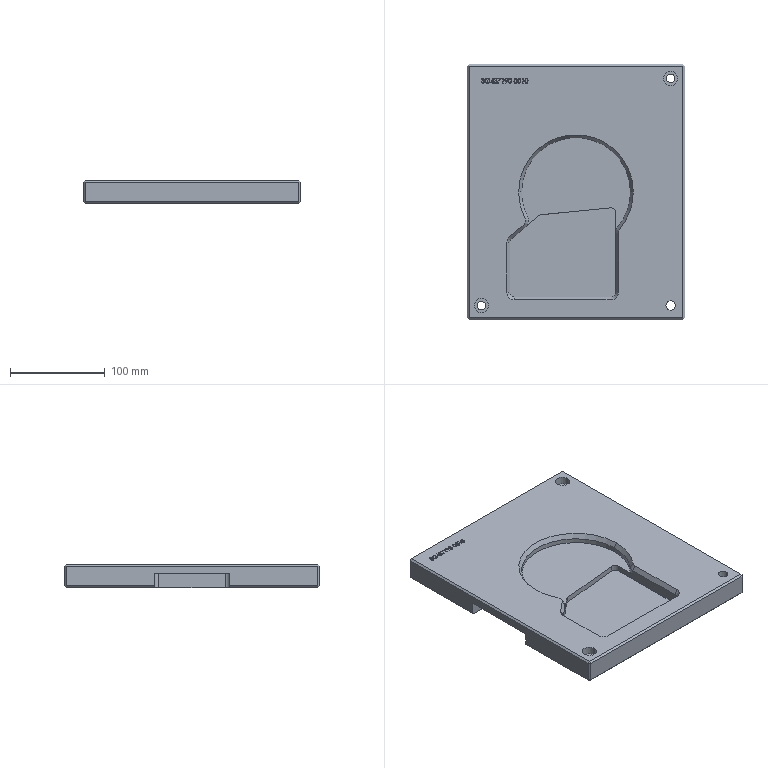Part | STEP file | Market locating fixture base plate | 1 solid | 237 faces | box 230 x 270 x 25 mm | volume 1234801 mm3 | plane 115 | spline 83 | cylinder 25 | cone 14 | commonest cylinder face diameters 10 x11 9 x4 15 x4 20 x3 115 x3